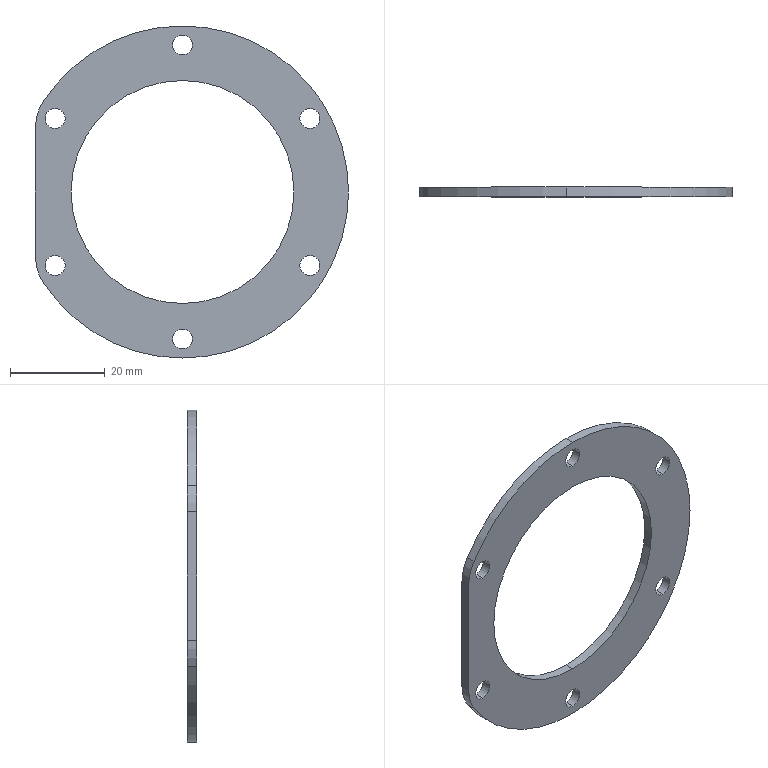Part | SolidWorks | features Extrusion 1 | 1 solid | 22 faces | box 66 x 2 x 70 mm | volume 3883 mm3 | cylinder 19 | plane 3 | commonest cylinder face diameters 4.2 x12 70 x3 20 x2 47 x2
STEP:
#1=CARTESIAN_POINT('',(-26.847,2.,-17.6));
#2=VERTEX_POINT('',#1);
#3=CARTESIAN_POINT('',(-26.847,2.,-13.4));
#4=VERTEX_POINT('',#3);
#5=CARTESIAN_POINT('',(-26.847,2.,-15.5));
#6=DIRECTION('',(0.,1.,0.));
#7=DIRECTION('',(0.,0.,1.));
#8=AXIS2_PLACEMENT_3D('',#5,#6,#7);
#9=CIRCLE('',#8,2.1);
#10=EDGE_CURVE('',#2,#4,#9,.T.);
#11=ORIENTED_EDGE('',*,*,#10,.T.);
#12=CARTESIAN_POINT('',(-26.847,0.,-13.4));
#13=VERTEX_POINT('',#12);
#14=CARTESIAN_POINT('',(-26.847,2.,-13.4));
#15=DIRECTION('',(0.,-1.,0.));
#16=VECTOR('',#15,1000.);
#17=LINE('',#14,#16);
#18=EDGE_CURVE('',#4,#13,#17,.T.);
#19=ORIENTED_EDGE('',*,*,#18,.T.);
#20=CARTESIAN_POINT('',(-26.847,0.,-17.6));
#21=VERTEX_POINT('',#20);
#22=CARTESIAN_POINT('',(-26.847,0.,-15.5));
#23=DIRECTION('',(0.,1.,0.));
#24=DIRECTION('',(0.,0.,1.));
#25=AXIS2_PLACEMENT_3D('',#22,#23,#24);
#26=CIRCLE('',#25,2.1);
#27=EDGE_CURVE('',#21,#13,#26,.T.);
#28=ORIENTED_EDGE('',*,*,#27,.F.);
#29=CARTESIAN_POINT('',(-26.847,2.,-17.6));
#30=DIRECTION('',(0.,-1.,0.));
#31=VECTOR('',#30,1000.);
#32=LINE('',#29,#31);
#33=EDGE_CURVE('',#2,#21,#32,.T.);
#34=ORIENTED_EDGE('',*,*,#33,.F.);
#35=EDGE_LOOP('',(#11,#19,#28,#34));
#36=FACE_OUTER_BOUND('',#35,.T.);
#37=CARTESIAN_POINT('',(-26.847,2.,-15.5));
#38=DIRECTION('',(0.,-1.,0.));
#39=DIRECTION('',(0.,0.,-1.));
#40=AXIS2_PLACEMENT_3D('',#37,#38,#39);
#41=CYLINDRICAL_SURFACE('',#40,2.1);
#42=ADVANCED_FACE('',(#36),#41,.F.);
#43=CARTESIAN_POINT('',(-26.847,2.,13.4));
#44=VERTEX_POINT('',#43);
#45=CARTESIAN_POINT('',(-26.847,2.,17.6));
#46=VERTEX_POINT('',#45);
#47=CARTESIAN_POINT('',(-26.847,2.,15.5));
#48=DIRECTION('',(0.,1.,0.));
#49=DIRECTION('',(0.,0.,1.));
#50=AXIS2_PLACEMENT_3D('',#47,#48,#49);
#51=CIRCLE('',#50,2.1);
#52=EDGE_CURVE('',#44,#46,#51,.T.);
#53=ORIENTED_EDGE('',*,*,#52,.T.);
#54=CARTESIAN_POINT('',(-26.847,0.,17.6));
#55=VERTEX_POINT('',#54);
#56=CARTESIAN_POINT('',(-26.847,2.,17.6));
#57=DIRECTION('',(0.,-1.,0.));
#58=VECTOR('',#57,1000.);
#59=LINE('',#56,#58);
#60=EDGE_CURVE('',#46,#55,#59,.T.);
#61=ORIENTED_EDGE('',*,*,#60,.T.);
#62=CARTESIAN_POINT('',(-26.847,0.,13.4));
#63=VERTEX_POINT('',#62);
#64=CARTESIAN_POINT('',(-26.847,0.,15.5));
#65=DIRECTION('',(0.,1.,0.));
#66=DIRECTION('',(0.,0.,1.));
#67=AXIS2_PLACEMENT_3D('',#64,#65,#66);
#68=CIRCLE('',#67,2.1);
#69=EDGE_CURVE('',#63,#55,#68,.T.);
#70=ORIENTED_EDGE('',*,*,#69,.F.);
#71=CARTESIAN_POINT('',(-26.847,2.,13.4));
#72=DIRECTION('',(0.,-1.,0.));
#73=VECTOR('',#72,1000.);
#74=LINE('',#71,#73);
#75=EDGE_CURVE('',#44,#63,#74,.T.);
#76=ORIENTED_EDGE('',*,*,#75,.F.);
#77=EDGE_LOOP('',(#53,#61,#70,#76));
#78=FACE_OUTER_BOUND('',#77,.T.);
#79=CARTESIAN_POINT('',(-26.847,2.,15.5));
#80=DIRECTION('',(0.,-1.,0.));
#81=DIRECTION('',(0.,0.,-1.));
#82=AXIS2_PLACEMENT_3D('',#79,#80,#81);
#83=CYLINDRICAL_SURFACE('',#82,2.1);
#84=ADVANCED_FACE('',(#78),#83,.F.);
#85=CARTESIAN_POINT('',(0.,2.,28.9));
#86=VERTEX_POINT('',#85);
#87=CARTESIAN_POINT('',(0.,2.,33.1));
#88=VERTEX_POINT('',#87);
#89=CARTESIAN_POINT('',(0.,2.,31.));
#90=DIRECTION('',(0.,1.,0.));
#91=DIRECTION('',(0.,0.,1.));
#92=AXIS2_PLACEMENT_3D('',#89,#90,#91);
#93=CIRCLE('',#92,2.1);
#94=EDGE_CURVE('',#86,#88,#93,.T.);
#95=ORIENTED_EDGE('',*,*,#94,.T.);
#96=CARTESIAN_POINT('',(0.,0.,33.1));
#97=VERTEX_POINT('',#96);
#98=CARTESIAN_POINT('',(0.,2.,33.1));
#99=DIRECTION('',(0.,-1.,0.));
#100=VECTOR('',#99,1000.);
#101=LINE('',#98,#100);
#102=EDGE_CURVE('',#88,#97,#101,.T.);
#103=ORIENTED_EDGE('',*,*,#102,.T.);
#104=CARTESIAN_POINT('',(0.,0.,28.9));
#105=VERTEX_POINT('',#104);
#106=CARTESIAN_POINT('',(0.,0.,31.));
#107=DIRECTION('',(0.,1.,0.));
#108=DIRECTION('',(0.,0.,1.));
#109=AXIS2_PLACEMENT_3D('',#106,#107,#108);
#110=CIRCLE('',#109,2.1);
#111=EDGE_CURVE('',#105,#97,#110,.T.);
#112=ORIENTED_EDGE('',*,*,#111,.F.);
#113=CARTESIAN_POINT('',(0.,2.,28.9));
#114=DIRECTION('',(0.,-1.,0.));
#115=VECTOR('',#114,1000.);
#116=LINE('',#113,#115);
#117=EDGE_CURVE('',#86,#105,#116,.T.);
#118=ORIENTED_EDGE('',*,*,#117,.F.);
#119=EDGE_LOOP('',(#95,#103,#112,#118));
#120=FACE_OUTER_BOUND('',#119,.T.);
#121=CARTESIAN_POINT('',(0.,2.,31.));
#122=DIRECTION('',(0.,-1.,0.));
#123=DIRECTION('',(0.,0.,-1.));
#124=AXIS2_PLACEMENT_3D('',#121,#122,#123);
#125=CYLINDRICAL_SURFACE('',#124,2.1);
#126=ADVANCED_FACE('',(#120),#125,.F.);
#127=CARTESIAN_POINT('',(26.847,2.,13.4));
#128=VERTEX_POINT('',#127);
#129=CARTESIAN_POINT('',(26.847,2.,17.6));
#130=VERTEX_POINT('',#129);
#131=CARTESIAN_POINT('',(26.847,2.,15.5));
#132=DIRECTION('',(0.,1.,0.));
#133=DIRECTION('',(0.,0.,1.));
#134=AXIS2_PLACEMENT_3D('',#131,#132,#133);
#135=CIRCLE('',#134,2.1);
#136=EDGE_CURVE('',#128,#130,#135,.T.);
#137=ORIENTED_EDGE('',*,*,#136,.T.);
#138=CARTESIAN_POINT('',(26.847,0.,17.6));
#139=VERTEX_POINT('',#138);
#140=CARTESIAN_POINT('',(26.847,2.,17.6));
#141=DIRECTION('',(0.,-1.,0.));
#142=VECTOR('',#141,1000.);
#143=LINE('',#140,#142);
#144=EDGE_CURVE('',#130,#139,#143,.T.);
#145=ORIENTED_EDGE('',*,*,#144,.T.);
#146=CARTESIAN_POINT('',(26.847,0.,13.4));
#147=VERTEX_POINT('',#146);
#148=CARTESIAN_POINT('',(26.847,0.,15.5));
#149=DIRECTION('',(0.,1.,0.));
#150=DIRECTION('',(0.,0.,1.));
#151=AXIS2_PLACEMENT_3D('',#148,#149,#150);
#152=CIRCLE('',#151,2.1);
#153=EDGE_CURVE('',#147,#139,#152,.T.);
#154=ORIENTED_EDGE('',*,*,#153,.F.);
#155=CARTESIAN_POINT('',(26.847,2.,13.4));
#156=DIRECTION('',(0.,-1.,0.));
#157=VECTOR('',#156,1000.);
#158=LINE('',#155,#157);
#159=EDGE_CURVE('',#128,#147,#158,.T.);
#160=ORIENTED_EDGE('',*,*,#159,.F.);
#161=EDGE_LOOP('',(#137,#145,#154,#160));
#162=FACE_OUTER_BOUND('',#161,.T.);
#163=CARTESIAN_POINT('',(26.847,2.,15.5));
#164=DIRECTION('',(0.,-1.,0.));
#165=DIRECTION('',(0.,0.,-1.));
#166=AXIS2_PLACEMENT_3D('',#163,#164,#165);
#167=CYLINDRICAL_SURFACE('',#166,2.1);
#168=ADVANCED_FACE('',(#162),#167,.F.);
#169=CARTESIAN_POINT('',(26.847,2.,-17.6));
#170=VERTEX_POINT('',#169);
#171=CARTESIAN_POINT('',(26.847,2.,-13.4));
#172=VERTEX_POINT('',#171);
#173=CARTESIAN_POINT('',(26.847,2.,-15.5));
#174=DIRECTION('',(0.,1.,0.));
#175=DIRECTION('',(0.,0.,1.));
#176=AXIS2_PLACEMENT_3D('',#173,#174,#175);
#177=CIRCLE('',#176,2.1);
#178=EDGE_CURVE('',#170,#172,#177,.T.);
#179=ORIENTED_EDGE('',*,*,#178,.T.);
#180=CARTESIAN_POINT('',(26.847,0.,-13.4));
#181=VERTEX_POINT('',#180);
#182=CARTESIAN_POINT('',(26.847,2.,-13.4));
#183=DIRECTION('',(0.,-1.,0.));
#184=VECTOR('',#183,1000.);
#185=LINE('',#182,#184);
#186=EDGE_CURVE('',#172,#181,#185,.T.);
#187=ORIENTED_EDGE('',*,*,#186,.T.);
#188=CARTESIAN_POINT('',(26.847,0.,-17.6));
#189=VERTEX_POINT('',#188);
#190=CARTESIAN_POINT('',(26.847,0.,-15.5));
#191=DIRECTION('',(0.,1.,0.));
#192=DIRECTION('',(0.,0.,1.));
#193=AXIS2_PLACEMENT_3D('',#190,#191,#192);
#194=CIRCLE('',#193,2.1);
#195=EDGE_CURVE('',#189,#181,#194,.T.);
#196=ORIENTED_EDGE('',*,*,#195,.F.);
#197=CARTESIAN_POINT('',(26.847,2.,-17.6));
#198=DIRECTION('',(0.,-1.,0.));
#199=VECTOR('',#198,1000.);
#200=LINE('',#197,#199);
#201=EDGE_CURVE('',#170,#189,#200,.T.);
#202=ORIENTED_EDGE('',*,*,#201,.F.);
#203=EDGE_LOOP('',(#179,#187,#196,#202));
#204=FACE_OUTER_BOUND('',#203,.T.);
#205=CARTESIAN_POINT('',(26.847,2.,-15.5));
#206=DIRECTION('',(0.,-1.,0.));
#207=DIRECTION('',(0.,0.,-1.));
#208=AXIS2_PLACEMENT_3D('',#205,#206,#207);
#209=CYLINDRICAL_SURFACE('',#208,2.1);
#210=ADVANCED_FACE('',(#204),#209,.F.);
#211=CARTESIAN_POINT('',(0.,2.,-33.1));
#212=VERTEX_POINT('',#211);
#213=CARTESIAN_POINT('',(0.,2.,-28.9));
#214=VERTEX_POINT('',#213);
#215=CARTESIAN_POINT('',(0.,2.,-31.));
#216=DIRECTION('',(0.,1.,0.));
#217=DIRECTION('',(0.,0.,1.));
#218=AXIS2_PLACEMENT_3D('',#215,#216,#217);
#219=CIRCLE('',#218,2.1);
#220=EDGE_CURVE('',#212,#214,#219,.T.);
#221=ORIENTED_EDGE('',*,*,#220,.T.);
#222=CARTESIAN_POINT('',(0.,0.,-28.9));
#223=VERTEX_POINT('',#222);
#224=CARTESIAN_POINT('',(0.,2.,-28.9));
#225=DIRECTION('',(0.,-1.,0.));
#226=VECTOR('',#225,1000.);
#227=LINE('',#224,#226);
#228=EDGE_CURVE('',#214,#223,#227,.T.);
#229=ORIENTED_EDGE('',*,*,#228,.T.);
#230=CARTESIAN_POINT('',(0.,0.,-33.1));
#231=VERTEX_POINT('',#230);
#232=CARTESIAN_POINT('',(0.,0.,-31.));
#233=DIRECTION('',(0.,1.,0.));
#234=DIRECTION('',(0.,0.,1.));
#235=AXIS2_PLACEMENT_3D('',#232,#233,#234);
#236=CIRCLE('',#235,2.1);
#237=EDGE_CURVE('',#231,#223,#236,.T.);
#238=ORIENTED_EDGE('',*,*,#237,.F.);
#239=CARTESIAN_POINT('',(0.,2.,-33.1));
#240=DIRECTION('',(0.,-1.,0.));
#241=VECTOR('',#240,1000.);
#242=LINE('',#239,#241);
#243=EDGE_CURVE('',#212,#231,#242,.T.);
#244=ORIENTED_EDGE('',*,*,#243,.F.);
#245=EDGE_LOOP('',(#221,#229,#238,#244));
#246=FACE_OUTER_BOUND('',#245,.T.);
#247=CARTESIAN_POINT('',(0.,2.,-31.));
#248=DIRECTION('',(0.,-1.,0.));
#249=DIRECTION('',(0.,0.,-1.));
#250=AXIS2_PLACEMENT_3D('',#247,#248,#249);
#251=CYLINDRICAL_SURFACE('',#250,2.1);
#252=ADVANCED_FACE('',(#246),#251,.F.);
#253=CARTESIAN_POINT('',(0.,2.,-23.5));
#254=VERTEX_POINT('',#253);
#255=CARTESIAN_POINT('',(0.,2.,23.5));
#256=VERTEX_POINT('',#255);
#257=CARTESIAN_POINT('',(0.,2.,0.));
#258=DIRECTION('',(0.,1.,0.));
#259=DIRECTION('',(0.,0.,1.));
#260=AXIS2_PLACEMENT_3D('',#257,#258,#259);
#261=CIRCLE('',#260,23.5);
#262=EDGE_CURVE('',#254,#256,#261,.T.);
#263=ORIENTED_EDGE('',*,*,#262,.T.);
#264=CARTESIAN_POINT('',(0.,0.,23.5));
#265=VERTEX_POINT('',#264);
#266=CARTESIAN_POINT('',(0.,2.,23.5));
#267=DIRECTION('',(0.,-1.,0.));
#268=VECTOR('',#267,1000.);
#269=LINE('',#266,#268);
#270=EDGE_CURVE('',#256,#265,#269,.T.);
#271=ORIENTED_EDGE('',*,*,#270,.T.);
#272=CARTESIAN_POINT('',(0.,0.,-23.5));
#273=VERTEX_POINT('',#272);
#274=CARTESIAN_POINT('',(0.,0.,0.));
#275=DIRECTION('',(0.,1.,0.));
#276=DIRECTION('',(0.,0.,1.));
#277=AXIS2_PLACEMENT_3D('',#274,#275,#276);
#278=CIRCLE('',#277,23.5);
#279=EDGE_CURVE('',#273,#265,#278,.T.);
#280=ORIENTED_EDGE('',*,*,#279,.F.);
#281=CARTESIAN_POINT('',(0.,2.,-23.5));
#282=DIRECTION('',(0.,-1.,0.));
#283=VECTOR('',#282,1000.);
#284=LINE('',#281,#283);
#285=EDGE_CURVE('',#254,#273,#284,.T.);
#286=ORIENTED_EDGE('',*,*,#285,.F.);
#287=EDGE_LOOP('',(#263,#271,#280,#286));
#288=FACE_OUTER_BOUND('',#287,.T.);
#289=CARTESIAN_POINT('',(0.,2.,0.));
#290=DIRECTION('',(0.,-1.,0.));
#291=DIRECTION('',(0.,0.,-1.));
#292=AXIS2_PLACEMENT_3D('',#289,#290,#291);
#293=CYLINDRICAL_SURFACE('',#292,23.5);
#294=ADVANCED_FACE('',(#288),#293,.F.);
#295=CARTESIAN_POINT('',(0.,2.,35.));
#296=VERTEX_POINT('',#295);
#297=CARTESIAN_POINT('',(0.,2.,-35.));
#298=VERTEX_POINT('',#297);
#299=CARTESIAN_POINT('',(0.,2.,0.));
#300=DIRECTION('',(0.,1.,0.));
#301=DIRECTION('',(0.,0.,1.));
#302=AXIS2_PLACEMENT_3D('',#299,#300,#301);
#303=CIRCLE('',#302,35.);
#304=EDGE_CURVE('',#296,#298,#303,.T.);
#305=ORIENTED_EDGE('',*,*,#304,.F.);
#306=CARTESIAN_POINT('',(0.,0.,35.));
#307=VERTEX_POINT('',#306);
#308=CARTESIAN_POINT('',(0.,2.,35.));
#309=DIRECTION('',(0.,-1.,0.));
#310=VECTOR('',#309,1000.);
#311=LINE('',#308,#310);
#312=EDGE_CURVE('',#296,#307,#311,.T.);
#313=ORIENTED_EDGE('',*,*,#312,.T.);
#314=CARTESIAN_POINT('',(0.,0.,-35.));
#315=VERTEX_POINT('',#314);
#316=CARTESIAN_POINT('',(0.,0.,0.));
#317=DIRECTION('',(0.,1.,0.));
#318=DIRECTION('',(0.,0.,1.));
#319=AXIS2_PLACEMENT_3D('',#316,#317,#318);
#320=CIRCLE('',#319,35.);
#321=EDGE_CURVE('',#307,#315,#320,.T.);
#322=ORIENTED_EDGE('',*,*,#321,.T.);
#323=CARTESIAN_POINT('',(0.,2.,-35.));
#324=DIRECTION('',(0.,-1.,0.));
#325=VECTOR('',#324,1000.);
#326=LINE('',#323,#325);
#327=EDGE_CURVE('',#298,#315,#326,.T.);
#328=ORIENTED_EDGE('',*,*,#327,.F.);
#329=EDGE_LOOP('',(#305,#313,#322,#328));
#330=FACE_OUTER_BOUND('',#329,.T.);
#331=CARTESIAN_POINT('',(0.,2.,0.));
#332=DIRECTION('',(0.,-1.,0.));
#333=DIRECTION('',(0.,0.,-1.));
#334=AXIS2_PLACEMENT_3D('',#331,#332,#333);
#335=CYLINDRICAL_SURFACE('',#334,35.);
#336=ADVANCED_FACE('',(#330),#335,.T.);
#337=CARTESIAN_POINT('',(-29.4,2.,-18.991));
#338=VERTEX_POINT('',#337);
#339=CARTESIAN_POINT('',(0.,2.,0.));
#340=DIRECTION('',(0.,1.,0.));
#341=DIRECTION('',(0.,0.,1.));
#342=AXIS2_PLACEMENT_3D('',#339,#340,#341);
#343=CIRCLE('',#342,35.);
#344=EDGE_CURVE('',#298,#338,#343,.T.);
#345=ORIENTED_EDGE('',*,*,#344,.F.);
#346=ORIENTED_EDGE('',*,*,#327,.T.);
#347=CARTESIAN_POINT('',(-29.4,0.,-18.991));
#348=VERTEX_POINT('',#347);
#349=CARTESIAN_POINT('',(0.,0.,0.));
#350=DIRECTION('',(0.,1.,0.));
#351=DIRECTION('',(0.,0.,1.));
#352=AXIS2_PLACEMENT_3D('',#349,#350,#351);
#353=CIRCLE('',#352,35.);
#354=EDGE_CURVE('',#315,#348,#353,.T.);
#355=ORIENTED_EDGE('',*,*,#354,.T.);
#356=CARTESIAN_POINT('',(-29.4,2.,-18.991));
#357=DIRECTION('',(0.,-1.,0.));
#358=VECTOR('',#357,1000.);
#359=LINE('',#356,#358);
#360=EDGE_CURVE('',#338,#348,#359,.T.);
#361=ORIENTED_EDGE('',*,*,#360,.F.);
#362=EDGE_LOOP('',(#345,#346,#355,#361));
#363=FACE_OUTER_BOUND('',#362,.T.);
#364=CARTESIAN_POINT('',(0.,2.,0.));
#365=DIRECTION('',(0.,-1.,0.));
#366=DIRECTION('',(0.,0.,-1.));
#367=AXIS2_PLACEMENT_3D('',#364,#365,#366);
#368=CYLINDRICAL_SURFACE('',#367,35.);
#369=ADVANCED_FACE('',(#363),#368,.T.);
#370=CARTESIAN_POINT('',(-31.,2.,13.565));
#371=VERTEX_POINT('',#370);
#372=CARTESIAN_POINT('',(-29.4,2.,18.991));
#373=VERTEX_POINT('',#372);
#374=CARTESIAN_POINT('',(-21.,2.,13.565));
#375=DIRECTION('',(0.,1.,0.));
#376=DIRECTION('',(0.,0.,-1.));
#377=AXIS2_PLACEMENT_3D('',#374,#375,#376);
#378=CIRCLE('',#377,10.);
#379=EDGE_CURVE('',#371,#373,#378,.T.);
#380=ORIENTED_EDGE('',*,*,#379,.T.);
#381=CARTESIAN_POINT('',(0.,2.,0.));
#382=DIRECTION('',(0.,1.,0.));
#383=DIRECTION('',(0.,0.,1.));
#384=AXIS2_PLACEMENT_3D('',#381,#382,#383);
#385=CIRCLE('',#384,35.);
#386=EDGE_CURVE('',#373,#296,#385,.T.);
#387=ORIENTED_EDGE('',*,*,#386,.T.);
#388=ORIENTED_EDGE('',*,*,#304,.T.);
#389=ORIENTED_EDGE('',*,*,#344,.T.);
#390=CARTESIAN_POINT('',(-31.,2.,-13.565));
#391=VERTEX_POINT('',#390);
#392=CARTESIAN_POINT('',(-21.,2.,-13.565));
#393=DIRECTION('',(0.,1.,0.));
#394=DIRECTION('',(0.,0.,-1.));
#395=AXIS2_PLACEMENT_3D('',#392,#393,#394);
#396=CIRCLE('',#395,10.);
#397=EDGE_CURVE('',#338,#391,#396,.T.);
#398=ORIENTED_EDGE('',*,*,#397,.T.);
#399=CARTESIAN_POINT('',(-31.,2.,13.565));
#400=DIRECTION('',(0.,0.,1.));
#401=VECTOR('',#400,1000.);
#402=LINE('',#399,#401);
#403=EDGE_CURVE('',#391,#371,#402,.T.);
#404=ORIENTED_EDGE('',*,*,#403,.T.);
#405=EDGE_LOOP('',(#380,#387,#388,#389,#398,#404));
#406=FACE_OUTER_BOUND('',#405,.T.);
#407=ORIENTED_EDGE('',*,*,#262,.F.);
#408=CARTESIAN_POINT('',(0.,2.,0.));
#409=DIRECTION('',(0.,1.,0.));
#410=DIRECTION('',(0.,0.,1.));
#411=AXIS2_PLACEMENT_3D('',#408,#409,#410);
#412=CIRCLE('',#411,23.5);
#413=EDGE_CURVE('',#256,#254,#412,.T.);
#414=ORIENTED_EDGE('',*,*,#413,.F.);
#415=EDGE_LOOP('',(#407,#414));
#416=FACE_BOUND('',#415,.T.);
#417=ORIENTED_EDGE('',*,*,#220,.F.);
#418=CARTESIAN_POINT('',(0.,2.,-31.));
#419=DIRECTION('',(0.,1.,0.));
#420=DIRECTION('',(0.,0.,1.));
#421=AXIS2_PLACEMENT_3D('',#418,#419,#420);
#422=CIRCLE('',#421,2.1);
#423=EDGE_CURVE('',#214,#212,#422,.T.);
#424=ORIENTED_EDGE('',*,*,#423,.F.);
#425=EDGE_LOOP('',(#417,#424));
#426=FACE_BOUND('',#425,.T.);
#427=ORIENTED_EDGE('',*,*,#178,.F.);
#428=CARTESIAN_POINT('',(26.847,2.,-15.5));
#429=DIRECTION('',(0.,1.,0.));
#430=DIRECTION('',(0.,0.,1.));
#431=AXIS2_PLACEMENT_3D('',#428,#429,#430);
#432=CIRCLE('',#431,2.1);
#433=EDGE_CURVE('',#172,#170,#432,.T.);
#434=ORIENTED_EDGE('',*,*,#433,.F.);
#435=EDGE_LOOP('',(#427,#434));
#436=FACE_BOUND('',#435,.T.);
#437=ORIENTED_EDGE('',*,*,#136,.F.);
#438=CARTESIAN_POINT('',(26.847,2.,15.5));
#439=DIRECTION('',(0.,1.,0.));
#440=DIRECTION('',(0.,0.,1.));
#441=AXIS2_PLACEMENT_3D('',#438,#439,#440);
#442=CIRCLE('',#441,2.1);
#443=EDGE_CURVE('',#130,#128,#442,.T.);
#444=ORIENTED_EDGE('',*,*,#443,.F.);
#445=EDGE_LOOP('',(#437,#444));
#446=FACE_BOUND('',#445,.T.);
#447=ORIENTED_EDGE('',*,*,#94,.F.);
#448=CARTESIAN_POINT('',(0.,2.,31.));
#449=DIRECTION('',(0.,1.,0.));
#450=DIRECTION('',(0.,0.,1.));
#451=AXIS2_PLACEMENT_3D('',#448,#449,#450);
#452=CIRCLE('',#451,2.1);
#453=EDGE_CURVE('',#88,#86,#452,.T.);
#454=ORIENTED_EDGE('',*,*,#453,.F.);
#455=EDGE_LOOP('',(#447,#454));
#456=FACE_BOUND('',#455,.T.);
#457=ORIENTED_EDGE('',*,*,#52,.F.);
#458=CARTESIAN_POINT('',(-26.847,2.,15.5));
#459=DIRECTION('',(0.,1.,0.));
#460=DIRECTION('',(0.,0.,1.));
#461=AXIS2_PLACEMENT_3D('',#458,#459,#460);
#462=CIRCLE('',#461,2.1);
#463=EDGE_CURVE('',#46,#44,#462,.T.);
#464=ORIENTED_EDGE('',*,*,#463,.F.);
#465=EDGE_LOOP('',(#457,#464));
#466=FACE_BOUND('',#465,.T.);
#467=ORIENTED_EDGE('',*,*,#10,.F.);
#468=CARTESIAN_POINT('',(-26.847,2.,-15.5));
#469=DIRECTION('',(0.,1.,0.));
#470=DIRECTION('',(0.,0.,1.));
#471=AXIS2_PLACEMENT_3D('',#468,#469,#470);
#472=CIRCLE('',#471,2.1);
#473=EDGE_CURVE('',#4,#2,#472,.T.);
#474=ORIENTED_EDGE('',*,*,#473,.F.);
#475=EDGE_LOOP('',(#467,#474));
#476=FACE_BOUND('',#475,.T.);
#477=CARTESIAN_POINT('',(-21.,2.,13.565));
#478=DIRECTION('',(0.,-1.,0.));
#479=DIRECTION('',(0.,0.,-1.));
#480=AXIS2_PLACEMENT_3D('',#477,#478,#479);
#481=PLANE('',#480);
#482=ADVANCED_FACE('',(#406,#416,#426,#436,#446,#456,#466,#476),#481,.F.);
#483=ORIENTED_EDGE('',*,*,#69,.T.);
#484=CARTESIAN_POINT('',(-26.847,0.,15.5));
#485=DIRECTION('',(0.,1.,0.));
#486=DIRECTION('',(0.,0.,1.));
#487=AXIS2_PLACEMENT_3D('',#484,#485,#486);
#488=CIRCLE('',#487,2.1);
#489=EDGE_CURVE('',#55,#63,#488,.T.);
#490=ORIENTED_EDGE('',*,*,#489,.T.);
#491=EDGE_LOOP('',(#483,#490));
#492=FACE_BOUND('',#491,.T.);
#493=ORIENTED_EDGE('',*,*,#153,.T.);
#494=CARTESIAN_POINT('',(26.847,0.,15.5));
#495=DIRECTION('',(0.,1.,0.));
#496=DIRECTION('',(0.,0.,1.));
#497=AXIS2_PLACEMENT_3D('',#494,#495,#496);
#498=CIRCLE('',#497,2.1);
#499=EDGE_CURVE('',#139,#147,#498,.T.);
#500=ORIENTED_EDGE('',*,*,#499,.T.);
#501=EDGE_LOOP('',(#493,#500));
#502=FACE_BOUND('',#501,.T.);
#503=ORIENTED_EDGE('',*,*,#237,.T.);
#504=CARTESIAN_POINT('',(0.,0.,-31.));
#505=DIRECTION('',(0.,1.,0.));
#506=DIRECTION('',(0.,0.,1.));
#507=AXIS2_PLACEMENT_3D('',#504,#505,#506);
#508=CIRCLE('',#507,2.1);
#509=EDGE_CURVE('',#223,#231,#508,.T.);
#510=ORIENTED_EDGE('',*,*,#509,.T.);
#511=EDGE_LOOP('',(#503,#510));
#512=FACE_BOUND('',#511,.T.);
#513=CARTESIAN_POINT('',(-31.,0.,13.565));
#514=VERTEX_POINT('',#513);
#515=CARTESIAN_POINT('',(-29.4,0.,18.991));
#516=VERTEX_POINT('',#515);
#517=CARTESIAN_POINT('',(-21.,0.,13.565));
#518=DIRECTION('',(0.,1.,0.));
#519=DIRECTION('',(0.,0.,-1.));
#520=AXIS2_PLACEMENT_3D('',#517,#518,#519);
#521=CIRCLE('',#520,10.);
#522=EDGE_CURVE('',#514,#516,#521,.T.);
#523=ORIENTED_EDGE('',*,*,#522,.F.);
#524=CARTESIAN_POINT('',(-31.,0.,-13.565));
#525=VERTEX_POINT('',#524);
#526=CARTESIAN_POINT('',(-31.,0.,13.565));
#527=DIRECTION('',(0.,0.,1.));
#528=VECTOR('',#527,1000.);
#529=LINE('',#526,#528);
#530=EDGE_CURVE('',#525,#514,#529,.T.);
#531=ORIENTED_EDGE('',*,*,#530,.F.);
#532=CARTESIAN_POINT('',(-21.,0.,-13.565));
#533=DIRECTION('',(0.,1.,0.));
#534=DIRECTION('',(0.,0.,-1.));
#535=AXIS2_PLACEMENT_3D('',#532,#533,#534);
#536=CIRCLE('',#535,10.);
#537=EDGE_CURVE('',#348,#525,#536,.T.);
#538=ORIENTED_EDGE('',*,*,#537,.F.);
#539=ORIENTED_EDGE('',*,*,#354,.F.);
#540=ORIENTED_EDGE('',*,*,#321,.F.);
#541=CARTESIAN_POINT('',(0.,0.,0.));
#542=DIRECTION('',(0.,1.,0.));
#543=DIRECTION('',(0.,0.,1.));
#544=AXIS2_PLACEMENT_3D('',#541,#542,#543);
#545=CIRCLE('',#544,35.);
#546=EDGE_CURVE('',#516,#307,#545,.T.);
#547=ORIENTED_EDGE('',*,*,#546,.F.);
#548=EDGE_LOOP('',(#523,#531,#538,#539,#540,#547));
#549=FACE_OUTER_BOUND('',#548,.T.);
#550=ORIENTED_EDGE('',*,*,#279,.T.);
#551=CARTESIAN_POINT('',(0.,0.,0.));
#552=DIRECTION('',(0.,1.,0.));
#553=DIRECTION('',(0.,0.,1.));
#554=AXIS2_PLACEMENT_3D('',#551,#552,#553);
#555=CIRCLE('',#554,23.5);
#556=EDGE_CURVE('',#265,#273,#555,.T.);
#557=ORIENTED_EDGE('',*,*,#556,.T.);
#558=EDGE_LOOP('',(#550,#557));
#559=FACE_BOUND('',#558,.T.);
#560=ORIENTED_EDGE('',*,*,#195,.T.);
#561=CARTESIAN_POINT('',(26.847,0.,-15.5));
#562=DIRECTION('',(0.,1.,0.));
#563=DIRECTION('',(0.,0.,1.));
#564=AXIS2_PLACEMENT_3D('',#561,#562,#563);
#565=CIRCLE('',#564,2.1);
#566=EDGE_CURVE('',#181,#189,#565,.T.);
#567=ORIENTED_EDGE('',*,*,#566,.T.);
#568=EDGE_LOOP('',(#560,#567));
#569=FACE_BOUND('',#568,.T.);
#570=ORIENTED_EDGE('',*,*,#111,.T.);
#571=CARTESIAN_POINT('',(0.,0.,31.));
#572=DIRECTION('',(0.,1.,0.));
#573=DIRECTION('',(0.,0.,1.));
#574=AXIS2_PLACEMENT_3D('',#571,#572,#573);
#575=CIRCLE('',#574,2.1);
#576=EDGE_CURVE('',#97,#105,#575,.T.);
#577=ORIENTED_EDGE('',*,*,#576,.T.);
#578=EDGE_LOOP('',(#570,#577));
#579=FACE_BOUND('',#578,.T.);
#580=ORIENTED_EDGE('',*,*,#27,.T.);
#581=CARTESIAN_POINT('',(-26.847,0.,-15.5));
#582=DIRECTION('',(0.,1.,0.));
#583=DIRECTION('',(0.,0.,1.));
#584=AXIS2_PLACEMENT_3D('',#581,#582,#583);
#585=CIRCLE('',#584,2.1);
#586=EDGE_CURVE('',#13,#21,#585,.T.);
#587=ORIENTED_EDGE('',*,*,#586,.T.);
#588=EDGE_LOOP('',(#580,#587));
#589=FACE_BOUND('',#588,.T.);
#590=CARTESIAN_POINT('',(-21.,0.,13.565));
#591=DIRECTION('',(0.,-1.,0.));
#592=DIRECTION('',(0.,0.,-1.));
#593=AXIS2_PLACEMENT_3D('',#590,#591,#592);
#594=PLANE('',#593);
#595=ADVANCED_FACE('',(#492,#502,#512,#549,#559,#569,#579,#589),#594,.T.);
#596=ORIENTED_EDGE('',*,*,#522,.T.);
#597=CARTESIAN_POINT('',(-29.4,2.,18.991));
#598=DIRECTION('',(0.,-1.,0.));
#599=VECTOR('',#598,1000.);
#600=LINE('',#597,#599);
#601=EDGE_CURVE('',#373,#516,#600,.T.);
#602=ORIENTED_EDGE('',*,*,#601,.F.);
#603=ORIENTED_EDGE('',*,*,#379,.F.);
#604=CARTESIAN_POINT('',(-31.,2.,13.565));
#605=DIRECTION('',(0.,-1.,0.));
#606=VECTOR('',#605,1000.);
#607=LINE('',#604,#606);
#608=EDGE_CURVE('',#371,#514,#607,.T.);
#609=ORIENTED_EDGE('',*,*,#608,.T.);
#610=EDGE_LOOP('',(#596,#602,#603,#609));
#611=FACE_OUTER_BOUND('',#610,.T.);
#612=CARTESIAN_POINT('',(-21.,2.,13.565));
#613=DIRECTION('',(0.,-1.,0.));
#614=DIRECTION('',(0.,0.,-1.));
#615=AXIS2_PLACEMENT_3D('',#612,#613,#614);
#616=CYLINDRICAL_SURFACE('',#615,10.);
#617=ADVANCED_FACE('',(#611),#616,.T.);
#618=ORIENTED_EDGE('',*,*,#312,.F.);
#619=ORIENTED_EDGE('',*,*,#386,.F.);
#620=ORIENTED_EDGE('',*,*,#601,.T.);
#621=ORIENTED_EDGE('',*,*,#546,.T.);
#622=EDGE_LOOP('',(#618,#619,#620,#621));
#623=FACE_OUTER_BOUND('',#622,.T.);
#624=CARTESIAN_POINT('',(0.,2.,0.));
#625=DIRECTION('',(0.,-1.,0.));
#626=DIRECTION('',(0.,0.,-1.));
#627=AXIS2_PLACEMENT_3D('',#624,#625,#626);
#628=CYLINDRICAL_SURFACE('',#627,35.);
#629=ADVANCED_FACE('',(#623),#628,.T.);
#630=ORIENTED_EDGE('',*,*,#537,.T.);
#631=CARTESIAN_POINT('',(-31.,2.,-13.565));
#632=DIRECTION('',(0.,-1.,0.));
#633=VECTOR('',#632,1000.);
#634=LINE('',#631,#633);
#635=EDGE_CURVE('',#391,#525,#634,.T.);
#636=ORIENTED_EDGE('',*,*,#635,.F.);
#637=ORIENTED_EDGE('',*,*,#397,.F.);
#638=ORIENTED_EDGE('',*,*,#360,.T.);
#639=EDGE_LOOP('',(#630,#636,#637,#638));
#640=FACE_OUTER_BOUND('',#639,.T.);
#641=CARTESIAN_POINT('',(-21.,2.,-13.565));
#642=DIRECTION('',(0.,-1.,0.));
#643=DIRECTION('',(0.,0.,-1.));
#644=AXIS2_PLACEMENT_3D('',#641,#642,#643);
#645=CYLINDRICAL_SURFACE('',#644,10.);
#646=ADVANCED_FACE('',(#640),#645,.T.);
#647=ORIENTED_EDGE('',*,*,#530,.T.);
#648=ORIENTED_EDGE('',*,*,#608,.F.);
#649=ORIENTED_EDGE('',*,*,#403,.F.);
#650=ORIENTED_EDGE('',*,*,#635,.T.);
#651=EDGE_LOOP('',(#647,#648,#649,#650));
#652=FACE_OUTER_BOUND('',#651,.T.);
#653=CARTESIAN_POINT('',(-31.,2.,13.565));
#654=DIRECTION('',(1.,0.,0.));
#655=DIRECTION('',(0.,0.,-1.));
#656=AXIS2_PLACEMENT_3D('',#653,#654,#655);
#657=PLANE('',#656);
#658=ADVANCED_FACE('',(#652),#657,.F.);
#659=ORIENTED_EDGE('',*,*,#270,.F.);
#660=ORIENTED_EDGE('',*,*,#413,.T.);
#661=ORIENTED_EDGE('',*,*,#285,.T.);
#662=ORIENTED_EDGE('',*,*,#556,.F.);
#663=EDGE_LOOP('',(#659,#660,#661,#662));
#664=FACE_OUTER_BOUND('',#663,.T.);
#665=CARTESIAN_POINT('',(0.,2.,0.));
#666=DIRECTION('',(0.,-1.,0.));
#667=DIRECTION('',(0.,0.,-1.));
#668=AXIS2_PLACEMENT_3D('',#665,#666,#667);
#669=CYLINDRICAL_SURFACE('',#668,23.5);
#670=ADVANCED_FACE('',(#664),#669,.F.);
#671=ORIENTED_EDGE('',*,*,#228,.F.);
#672=ORIENTED_EDGE('',*,*,#423,.T.);
#673=ORIENTED_EDGE('',*,*,#243,.T.);
#674=ORIENTED_EDGE('',*,*,#509,.F.);
#675=EDGE_LOOP('',(#671,#672,#673,#674));
#676=FACE_OUTER_BOUND('',#675,.T.);
#677=CARTESIAN_POINT('',(0.,2.,-31.));
#678=DIRECTION('',(0.,-1.,0.));
#679=DIRECTION('',(0.,0.,-1.));
#680=AXIS2_PLACEMENT_3D('',#677,#678,#679);
#681=CYLINDRICAL_SURFACE('',#680,2.1);
#682=ADVANCED_FACE('',(#676),#681,.F.);
#683=ORIENTED_EDGE('',*,*,#186,.F.);
#684=ORIENTED_EDGE('',*,*,#433,.T.);
#685=ORIENTED_EDGE('',*,*,#201,.T.);
#686=ORIENTED_EDGE('',*,*,#566,.F.);
#687=EDGE_LOOP('',(#683,#684,#685,#686));
#688=FACE_OUTER_BOUND('',#687,.T.);
#689=CARTESIAN_POINT('',(26.847,2.,-15.5));
#690=DIRECTION('',(0.,-1.,0.));
#691=DIRECTION('',(0.,0.,-1.));
#692=AXIS2_PLACEMENT_3D('',#689,#690,#691);
#693=CYLINDRICAL_SURFACE('',#692,2.1);
#694=ADVANCED_FACE('',(#688),#693,.F.);
#695=ORIENTED_EDGE('',*,*,#144,.F.);
#696=ORIENTED_EDGE('',*,*,#443,.T.);
#697=ORIENTED_EDGE('',*,*,#159,.T.);
#698=ORIENTED_EDGE('',*,*,#499,.F.);
#699=EDGE_LOOP('',(#695,#696,#697,#698));
#700=FACE_OUTER_BOUND('',#699,.T.);
#701=CARTESIAN_POINT('',(26.847,2.,15.5));
#702=DIRECTION('',(0.,-1.,0.));
#703=DIRECTION('',(0.,0.,-1.));
#704=AXIS2_PLACEMENT_3D('',#701,#702,#703);
#705=CYLINDRICAL_SURFACE('',#704,2.1);
#706=ADVANCED_FACE('',(#700),#705,.F.);
#707=ORIENTED_EDGE('',*,*,#102,.F.);
#708=ORIENTED_EDGE('',*,*,#453,.T.);
#709=ORIENTED_EDGE('',*,*,#117,.T.);
#710=ORIENTED_EDGE('',*,*,#576,.F.);
#711=EDGE_LOOP('',(#707,#708,#709,#710));
#712=FACE_OUTER_BOUND('',#711,.T.);
#713=CARTESIAN_POINT('',(0.,2.,31.));
#714=DIRECTION('',(0.,-1.,0.));
#715=DIRECTION('',(0.,0.,-1.));
#716=AXIS2_PLACEMENT_3D('',#713,#714,#715);
#717=CYLINDRICAL_SURFACE('',#716,2.1);
#718=ADVANCED_FACE('',(#712),#717,.F.);
#719=ORIENTED_EDGE('',*,*,#60,.F.);
#720=ORIENTED_EDGE('',*,*,#463,.T.);
#721=ORIENTED_EDGE('',*,*,#75,.T.);
#722=ORIENTED_EDGE('',*,*,#489,.F.);
#723=EDGE_LOOP('',(#719,#720,#721,#722));
#724=FACE_OUTER_BOUND('',#723,.T.);
#725=CARTESIAN_POINT('',(-26.847,2.,15.5));
#726=DIRECTION('',(0.,-1.,0.));
#727=DIRECTION('',(0.,0.,-1.));
#728=AXIS2_PLACEMENT_3D('',#725,#726,#727);
#729=CYLINDRICAL_SURFACE('',#728,2.1);
#730=ADVANCED_FACE('',(#724),#729,.F.);
#731=ORIENTED_EDGE('',*,*,#18,.F.);
#732=ORIENTED_EDGE('',*,*,#473,.T.);
#733=ORIENTED_EDGE('',*,*,#33,.T.);
#734=ORIENTED_EDGE('',*,*,#586,.F.);
#735=EDGE_LOOP('',(#731,#732,#733,#734));
#736=FACE_OUTER_BOUND('',#735,.T.);
#737=CARTESIAN_POINT('',(-26.847,2.,-15.5));
#738=DIRECTION('',(0.,-1.,0.));
#739=DIRECTION('',(0.,0.,-1.));
#740=AXIS2_PLACEMENT_3D('',#737,#738,#739);
#741=CYLINDRICAL_SURFACE('',#740,2.1);
#742=ADVANCED_FACE('',(#736),#741,.F.);
#743=CLOSED_SHELL('',(#42,#84,#126,#168,#210,#252,#294,#336,#369,#482,#595,#617,#629,#646,#658,#670,#682,#694,#706,#718,#730,#742));
#744=MANIFOLD_SOLID_BREP('',#743);
#745=CARTESIAN_POINT('',(0.,0.,0.));
#746=DIRECTION('',(0.,0.,1.));
#747=DIRECTION('',(1.,0.,0.));
#748=AXIS2_PLACEMENT_3D('',#745,#746,#747);
#749=(LENGTH_UNIT()NAMED_UNIT(*)SI_UNIT(.MILLI.,.METRE.));
#750=UNCERTAINTY_MEASURE_WITH_UNIT(LENGTH_MEASURE(0.00001),#749,'','');
#751=(NAMED_UNIT(*)PLANE_ANGLE_UNIT()SI_UNIT($,.RADIAN.));
#752=(NAMED_UNIT(*)SI_UNIT($,.STERADIAN.)SOLID_ANGLE_UNIT());
#753=(GEOMETRIC_REPRESENTATION_CONTEXT(3)GLOBAL_UNCERTAINTY_ASSIGNED_CONTEXT((#750))GLOBAL_UNIT_ASSIGNED_CONTEXT((#749,#751,#752))REPRESENTATION_CONTEXT('',''));
#754=ADVANCED_BREP_SHAPE_REPRESENTATION('',(#744,#748),#753);